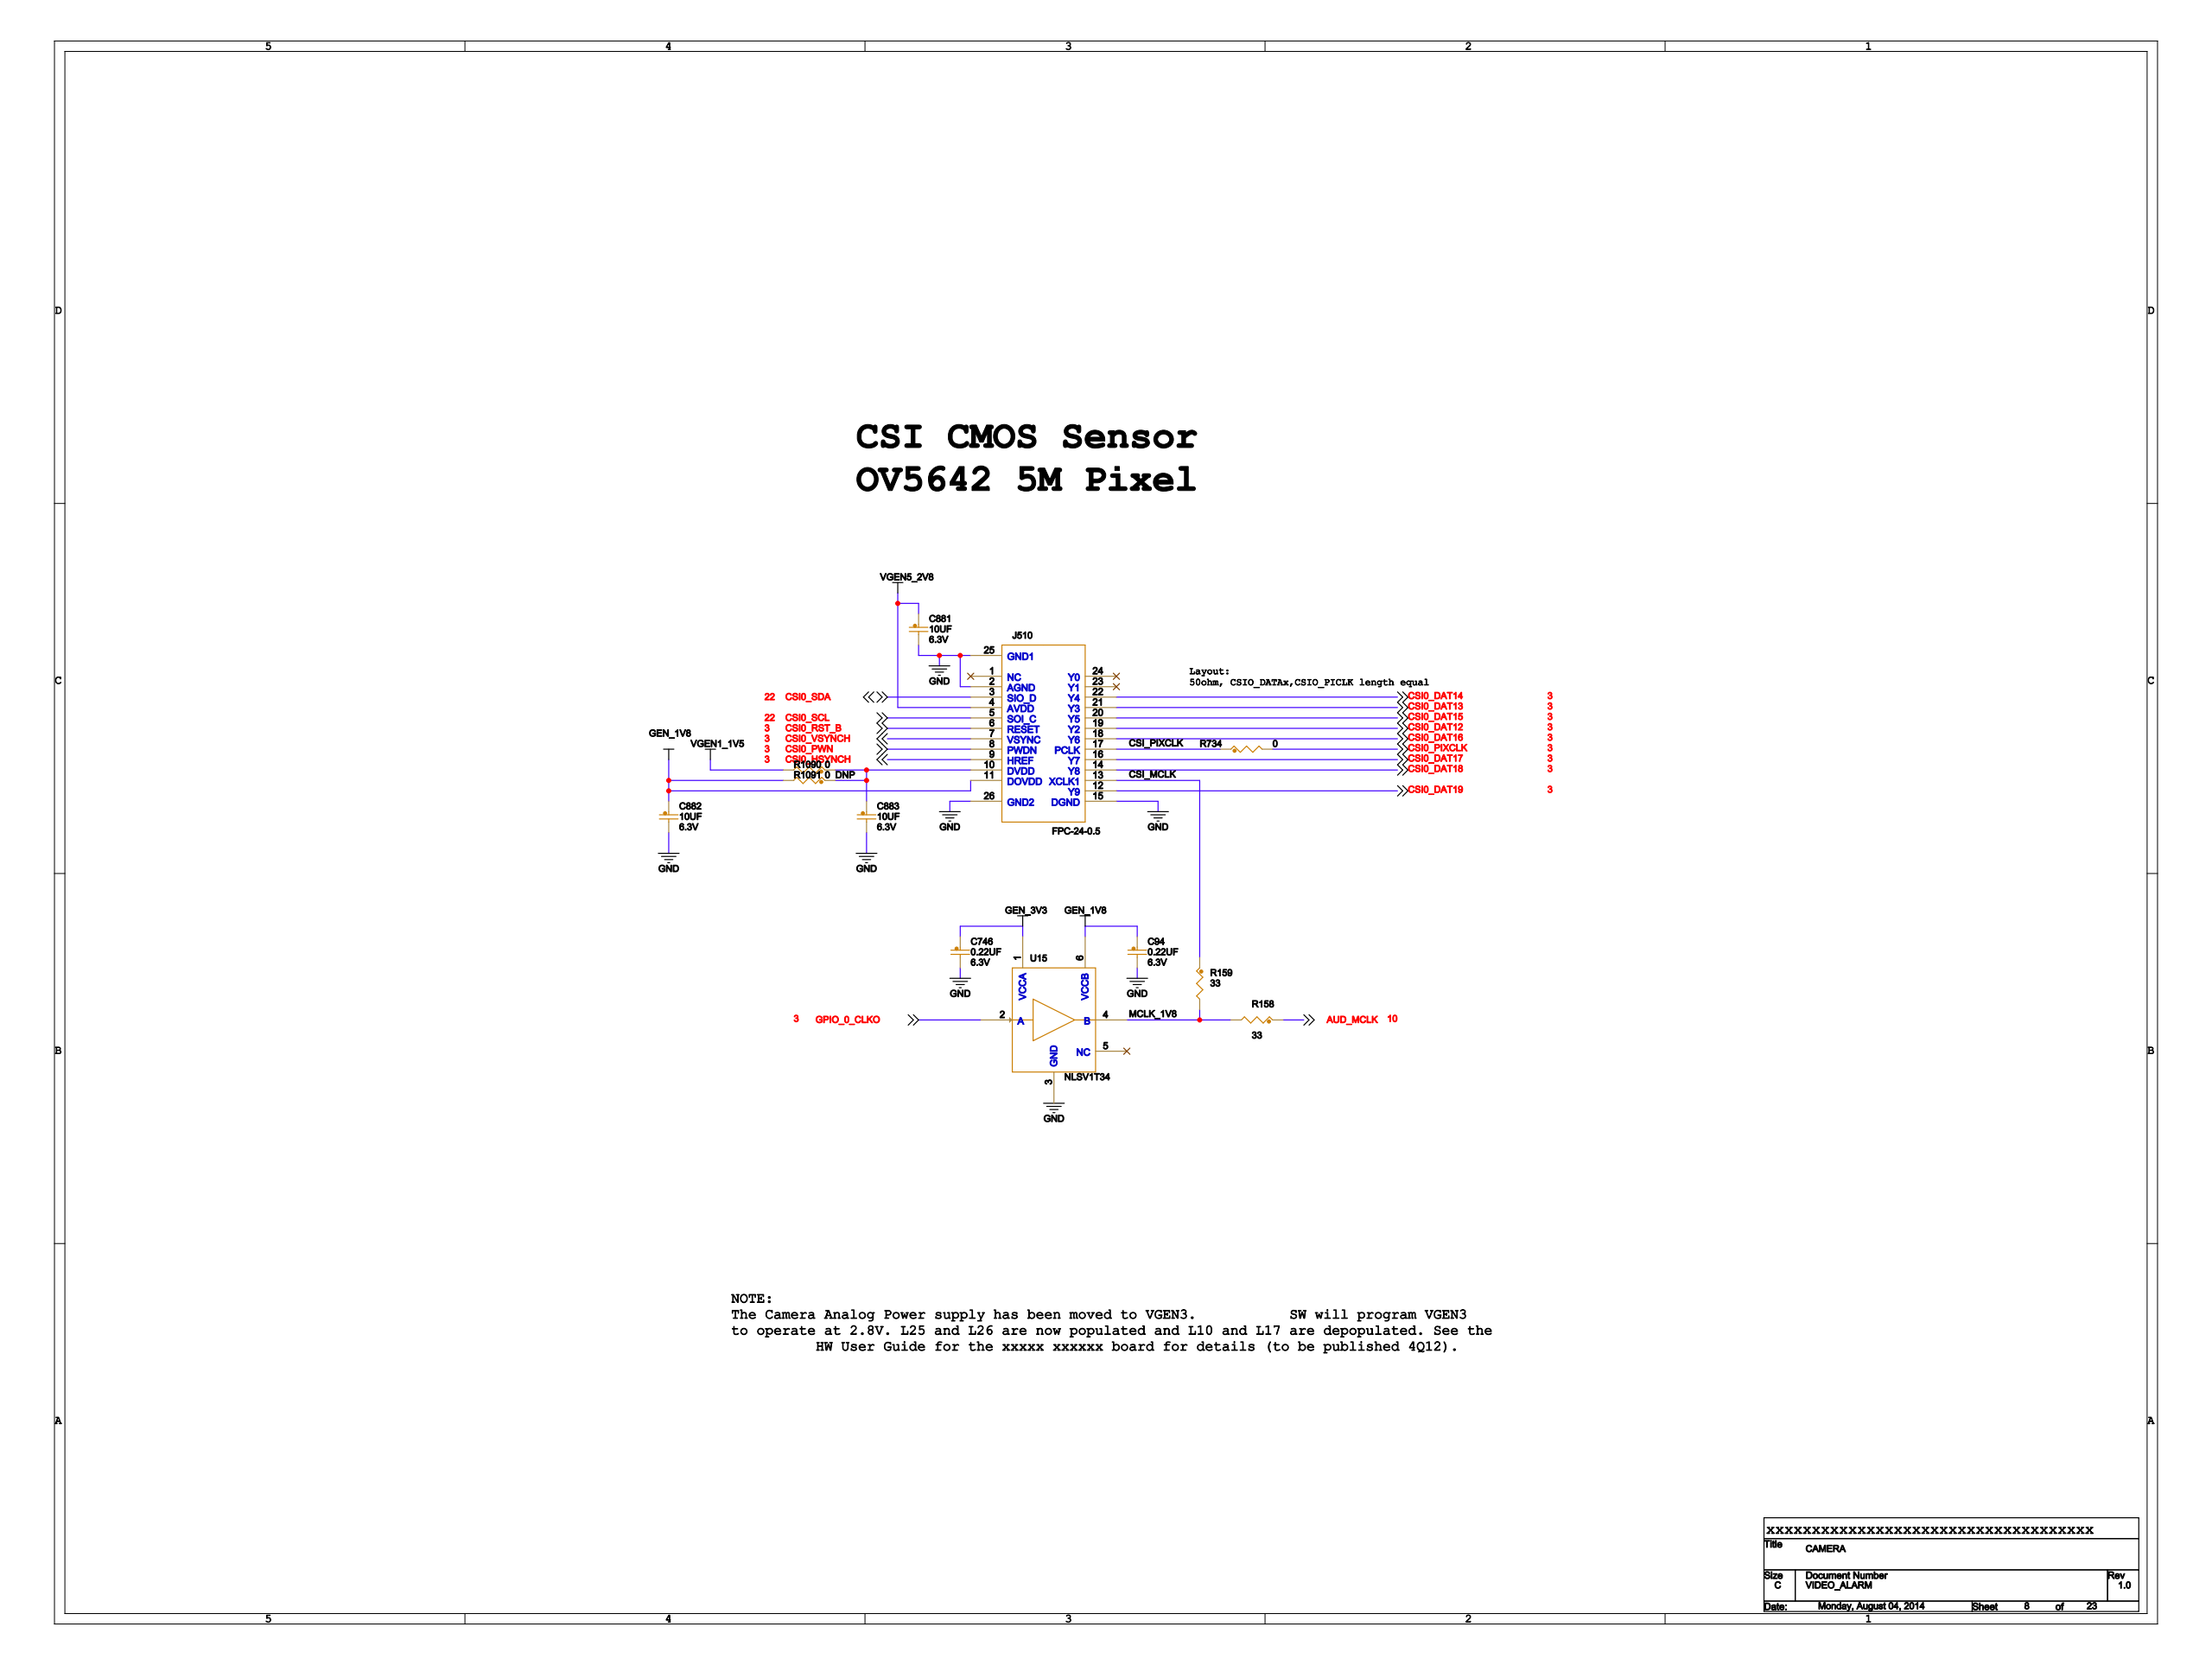Circuit board | Cadence Allegro | 994 parts | 728 nets | one sheet of the schematic
Parts on this sheet (reference | value | footprint):
C94 | 0.22UF | 0603_CC
C746 | 0.22UF | 0603_CC
C881 | 10UF | 0603_CC
C882 | 10UF | 0603_CC
C883 | 10UF | 0603_CC
J510 | FPC-24-0.5 | OV5642
R158 | 33 | 0603_CC
R159 | 33 | 0603_CC
R734 | 0 | 0603_CC
R1090 | 0 | 0603_CC
R1091 | 0 | 0603_CC
U15 | NLSV1T34 | ULLGA6_1P45X1_0P5MM
Nets of these parts (net: part-pin ...):
GND: C94-2 C746-2 C881-2 C882-2 C883-2 U15-3 J510-2 J510-15 J510-25 J510-26
GEN_3V3: C746-1 U15-1
VGEN1_1V5: R1090-2
VGEN5_2V8: C881-1 J510-4
GEN_1V8: C94-1 C882-1 R1091-2 U15-6 J510-11
CSI0_SDA: J510-3
CSI0_SCL: J510-5
CSI0_RST_B: J510-6
CSI0_VSYNCH: J510-7
CSI0_PWN: J510-8
CSI0_HSYNCH: J510-9
N22473908: C883-1 R1090-1 R1091-1 J510-10
CSI0_DAT19: J510-12
CSI_MCLK: R159-1 J510-13
CSI0_DAT18: J510-14
CSI0_DAT17: J510-16
CSI_PIXCLK: R734-1 J510-17
CSI0_DAT16: J510-18
CSI0_DAT12: J510-19
CSI0_DAT15: J510-20
CSI0_DAT13: J510-21
CSI0_DAT14: J510-22
MCLK_1V8: R158-2 R159-2 U15-4
AUD_MCLK: R158-1
CSI0_PIXCLK: R734-2
GPIO_0_CLKO: U15-2